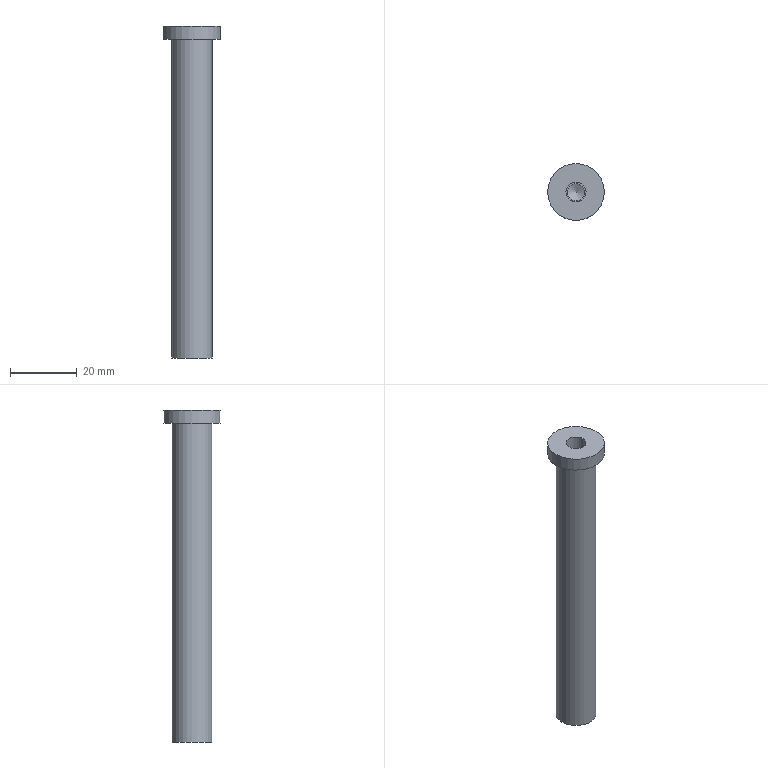Part | STEP file | solid 36 | 1 solid | 9 faces | box 17 x 17 x 99.469 mm | volume 11303 mm3 | plane 4 | cylinder 4 | cone 1 | commonest cylinder face diameters 5.1 x1 6 x1 12 x1 17 x1